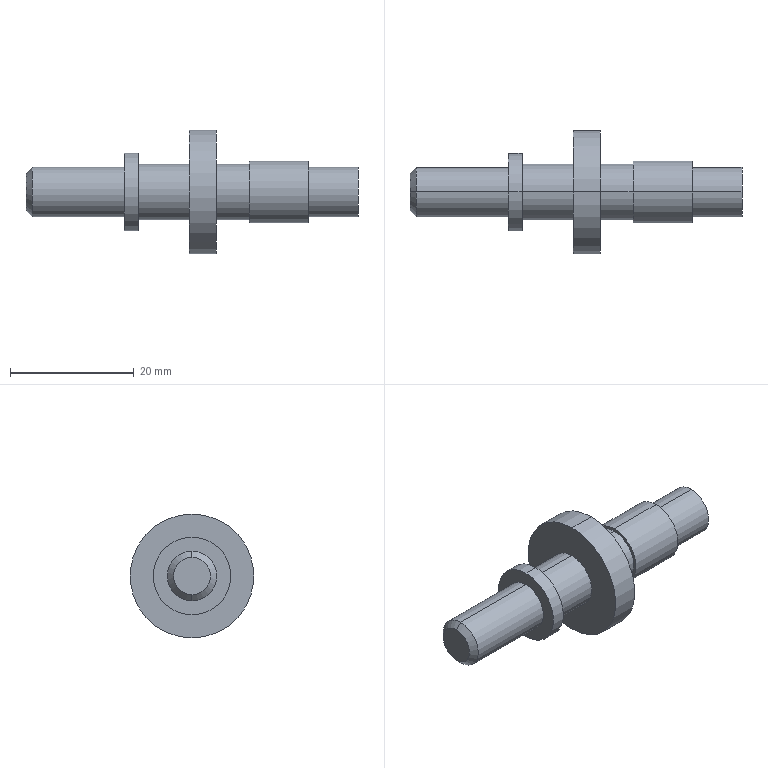Part | SolidWorks | features Revolution 1 | 1 solid | 25 faces | box 53.633 x 20 x 20 mm | volume 4453 mm3 | cylinder 14 | plane 7 | cone 4 | commonest cylinder face diameters 9 x4 8 x2 8.009 x2 10 x2 12.538 x2 20 x2
STEP:
#1=CARTESIAN_POINT('',(49.517,-18.474,-4.005));
#2=VERTEX_POINT('',#1);
#3=CARTESIAN_POINT('',(49.517,-18.474,4.005));
#4=VERTEX_POINT('',#3);
#5=CARTESIAN_POINT('',(49.517,-18.474,0.));
#6=DIRECTION('',(1.,0.,0.));
#7=DIRECTION('',(0.,0.,-1.));
#8=AXIS2_PLACEMENT_3D('',#5,#6,#7);
#9=CIRCLE('',#8,4.005);
#10=EDGE_CURVE('',#2,#4,#9,.T.);
#11=ORIENTED_EDGE('',*,*,#10,.F.);
#12=CARTESIAN_POINT('',(49.513,-18.474,-5.));
#13=VERTEX_POINT('',#12);
#14=CARTESIAN_POINT('',(49.517,-18.474,-4.005));
#15=DIRECTION('',(-0.003804,0.,-1.));
#16=VECTOR('',#15,1000.);
#17=LINE('',#14,#16);
#18=EDGE_CURVE('',#2,#13,#17,.T.);
#19=ORIENTED_EDGE('',*,*,#18,.T.);
#20=CARTESIAN_POINT('',(49.513,-18.474,5.));
#21=VERTEX_POINT('',#20);
#22=CARTESIAN_POINT('',(49.513,-18.474,0.));
#23=DIRECTION('',(1.,0.,0.));
#24=DIRECTION('',(0.,0.,-1.));
#25=AXIS2_PLACEMENT_3D('',#22,#23,#24);
#26=CIRCLE('',#25,5.);
#27=EDGE_CURVE('',#13,#21,#26,.T.);
#28=ORIENTED_EDGE('',*,*,#27,.T.);
#29=CARTESIAN_POINT('',(49.517,-18.474,4.005));
#30=DIRECTION('',(-0.003804,0.,1.));
#31=VECTOR('',#30,1000.);
#32=LINE('',#29,#31);
#33=EDGE_CURVE('',#4,#21,#32,.T.);
#34=ORIENTED_EDGE('',*,*,#33,.F.);
#35=EDGE_LOOP('',(#11,#19,#28,#34));
#36=FACE_OUTER_BOUND('',#35,.T.);
#37=CARTESIAN_POINT('',(49.517,-18.474,0.));
#38=DIRECTION('',(-1.,0.,0.));
#39=DIRECTION('',(0.,0.,1.));
#40=AXIS2_PLACEMENT_3D('',#37,#38,#39);
#41=CONICAL_SURFACE('',#40,4.005,1.567);
#42=ADVANCED_FACE('',(#36),#41,.T.);
#43=ORIENTED_EDGE('',*,*,#10,.T.);
#44=CARTESIAN_POINT('',(57.517,-18.474,4.005));
#45=VERTEX_POINT('',#44);
#46=CARTESIAN_POINT('',(3.884,-18.474,4.005));
#47=DIRECTION('',(1.,0.,0.));
#48=VECTOR('',#47,1000.);
#49=LINE('',#46,#48);
#50=EDGE_CURVE('',#4,#45,#49,.T.);
#51=ORIENTED_EDGE('',*,*,#50,.T.);
#52=CARTESIAN_POINT('',(57.517,-18.474,-4.005));
#53=VERTEX_POINT('',#52);
#54=CARTESIAN_POINT('',(57.517,-18.474,0.));
#55=DIRECTION('',(1.,0.,0.));
#56=DIRECTION('',(0.,0.,-1.));
#57=AXIS2_PLACEMENT_3D('',#54,#55,#56);
#58=CIRCLE('',#57,4.005);
#59=EDGE_CURVE('',#53,#45,#58,.T.);
#60=ORIENTED_EDGE('',*,*,#59,.F.);
#61=CARTESIAN_POINT('',(3.884,-18.474,-4.005));
#62=DIRECTION('',(1.,0.,0.));
#63=VECTOR('',#62,1000.);
#64=LINE('',#61,#63);
#65=EDGE_CURVE('',#2,#53,#64,.T.);
#66=ORIENTED_EDGE('',*,*,#65,.F.);
#67=EDGE_LOOP('',(#43,#51,#60,#66));
#68=FACE_OUTER_BOUND('',#67,.T.);
#69=CARTESIAN_POINT('',(3.884,-18.474,0.));
#70=DIRECTION('',(1.,0.,0.));
#71=DIRECTION('',(0.,0.,-1.));
#72=AXIS2_PLACEMENT_3D('',#69,#70,#71);
#73=CYLINDRICAL_SURFACE('',#72,4.005);
#74=ADVANCED_FACE('',(#68),#73,.T.);
#75=CARTESIAN_POINT('',(3.884,-18.474,-3.));
#76=VERTEX_POINT('',#75);
#77=CARTESIAN_POINT('',(3.884,-18.474,3.));
#78=VERTEX_POINT('',#77);
#79=CARTESIAN_POINT('',(3.884,-18.474,0.));
#80=DIRECTION('',(1.,0.,0.));
#81=DIRECTION('',(0.,0.,-1.));
#82=AXIS2_PLACEMENT_3D('',#79,#80,#81);
#83=CIRCLE('',#82,3.);
#84=EDGE_CURVE('',#76,#78,#83,.T.);
#85=ORIENTED_EDGE('',*,*,#84,.T.);
#86=CARTESIAN_POINT('',(4.884,-18.474,4.));
#87=VERTEX_POINT('',#86);
#88=CARTESIAN_POINT('',(4.884,-18.474,4.));
#89=DIRECTION('',(0.7071,0.,0.7071));
#90=VECTOR('',#89,1000.);
#91=LINE('',#88,#90);
#92=EDGE_CURVE('',#78,#87,#91,.T.);
#93=ORIENTED_EDGE('',*,*,#92,.T.);
#94=CARTESIAN_POINT('',(4.884,-18.474,-4.));
#95=VERTEX_POINT('',#94);
#96=CARTESIAN_POINT('',(4.884,-18.474,0.));
#97=DIRECTION('',(1.,0.,0.));
#98=DIRECTION('',(0.,0.,-1.));
#99=AXIS2_PLACEMENT_3D('',#96,#97,#98);
#100=CIRCLE('',#99,4.);
#101=EDGE_CURVE('',#95,#87,#100,.T.);
#102=ORIENTED_EDGE('',*,*,#101,.F.);
#103=CARTESIAN_POINT('',(4.884,-18.474,-4.));
#104=DIRECTION('',(0.7071,0.,-0.7071));
#105=VECTOR('',#104,1000.);
#106=LINE('',#103,#105);
#107=EDGE_CURVE('',#76,#95,#106,.T.);
#108=ORIENTED_EDGE('',*,*,#107,.F.);
#109=EDGE_LOOP('',(#85,#93,#102,#108));
#110=FACE_OUTER_BOUND('',#109,.T.);
#111=CARTESIAN_POINT('',(4.884,-18.474,0.));
#112=DIRECTION('',(1.,0.,0.));
#113=DIRECTION('',(0.,0.,-1.));
#114=AXIS2_PLACEMENT_3D('',#111,#112,#113);
#115=CONICAL_SURFACE('',#114,4.,0.7854);
#116=ADVANCED_FACE('',(#110),#115,.T.);
#117=ORIENTED_EDGE('',*,*,#101,.T.);
#118=CARTESIAN_POINT('',(19.769,-18.474,4.));
#119=VERTEX_POINT('',#118);
#120=CARTESIAN_POINT('',(3.884,-18.474,4.));
#121=DIRECTION('',(1.,0.,0.));
#122=VECTOR('',#121,1000.);
#123=LINE('',#120,#122);
#124=EDGE_CURVE('',#87,#119,#123,.T.);
#125=ORIENTED_EDGE('',*,*,#124,.T.);
#126=CARTESIAN_POINT('',(19.769,-18.474,-4.));
#127=VERTEX_POINT('',#126);
#128=CARTESIAN_POINT('',(19.769,-18.474,0.));
#129=DIRECTION('',(1.,0.,0.));
#130=DIRECTION('',(0.,0.,-1.));
#131=AXIS2_PLACEMENT_3D('',#128,#129,#130);
#132=CIRCLE('',#131,4.);
#133=EDGE_CURVE('',#127,#119,#132,.T.);
#134=ORIENTED_EDGE('',*,*,#133,.F.);
#135=CARTESIAN_POINT('',(3.884,-18.474,-4.));
#136=DIRECTION('',(1.,0.,0.));
#137=VECTOR('',#136,1000.);
#138=LINE('',#135,#137);
#139=EDGE_CURVE('',#95,#127,#138,.T.);
#140=ORIENTED_EDGE('',*,*,#139,.F.);
#141=EDGE_LOOP('',(#117,#125,#134,#140));
#142=FACE_OUTER_BOUND('',#141,.T.);
#143=CARTESIAN_POINT('',(3.884,-18.474,0.));
#144=DIRECTION('',(1.,0.,0.));
#145=DIRECTION('',(0.,0.,-1.));
#146=AXIS2_PLACEMENT_3D('',#143,#144,#145);
#147=CYLINDRICAL_SURFACE('',#146,4.);
#148=ADVANCED_FACE('',(#142),#147,.T.);
#149=CARTESIAN_POINT('',(19.769,-18.474,-6.269));
#150=VERTEX_POINT('',#149);
#151=CARTESIAN_POINT('',(19.769,-18.474,6.269));
#152=VERTEX_POINT('',#151);
#153=CARTESIAN_POINT('',(19.769,-18.474,0.));
#154=DIRECTION('',(1.,0.,0.));
#155=DIRECTION('',(0.,0.,-1.));
#156=AXIS2_PLACEMENT_3D('',#153,#154,#155);
#157=CIRCLE('',#156,6.269);
#158=EDGE_CURVE('',#150,#152,#157,.T.);
#159=ORIENTED_EDGE('',*,*,#158,.T.);
#160=CARTESIAN_POINT('',(22.015,-18.474,6.269));
#161=VERTEX_POINT('',#160);
#162=CARTESIAN_POINT('',(3.884,-18.474,6.269));
#163=DIRECTION('',(1.,0.,0.));
#164=VECTOR('',#163,1000.);
#165=LINE('',#162,#164);
#166=EDGE_CURVE('',#152,#161,#165,.T.);
#167=ORIENTED_EDGE('',*,*,#166,.T.);
#168=CARTESIAN_POINT('',(22.015,-18.474,-6.269));
#169=VERTEX_POINT('',#168);
#170=CARTESIAN_POINT('',(22.015,-18.474,0.));
#171=DIRECTION('',(1.,0.,0.));
#172=DIRECTION('',(0.,0.,-1.));
#173=AXIS2_PLACEMENT_3D('',#170,#171,#172);
#174=CIRCLE('',#173,6.269);
#175=EDGE_CURVE('',#169,#161,#174,.T.);
#176=ORIENTED_EDGE('',*,*,#175,.F.);
#177=CARTESIAN_POINT('',(3.884,-18.474,-6.269));
#178=DIRECTION('',(1.,0.,0.));
#179=VECTOR('',#178,1000.);
#180=LINE('',#177,#179);
#181=EDGE_CURVE('',#150,#169,#180,.T.);
#182=ORIENTED_EDGE('',*,*,#181,.F.);
#183=EDGE_LOOP('',(#159,#167,#176,#182));
#184=FACE_OUTER_BOUND('',#183,.T.);
#185=CARTESIAN_POINT('',(3.884,-18.474,0.));
#186=DIRECTION('',(1.,0.,0.));
#187=DIRECTION('',(0.,0.,-1.));
#188=AXIS2_PLACEMENT_3D('',#185,#186,#187);
#189=CYLINDRICAL_SURFACE('',#188,6.269);
#190=ADVANCED_FACE('',(#184),#189,.T.);
#191=CARTESIAN_POINT('',(22.015,-18.474,-4.5));
#192=VERTEX_POINT('',#191);
#193=CARTESIAN_POINT('',(22.015,-18.474,4.5));
#194=VERTEX_POINT('',#193);
#195=CARTESIAN_POINT('',(22.015,-18.474,0.));
#196=DIRECTION('',(1.,0.,0.));
#197=DIRECTION('',(0.,0.,-1.));
#198=AXIS2_PLACEMENT_3D('',#195,#196,#197);
#199=CIRCLE('',#198,4.5);
#200=EDGE_CURVE('',#192,#194,#199,.T.);
#201=ORIENTED_EDGE('',*,*,#200,.T.);
#202=CARTESIAN_POINT('',(30.281,-18.474,4.5));
#203=VERTEX_POINT('',#202);
#204=CARTESIAN_POINT('',(3.884,-18.474,4.5));
#205=DIRECTION('',(1.,0.,0.));
#206=VECTOR('',#205,1000.);
#207=LINE('',#204,#206);
#208=EDGE_CURVE('',#194,#203,#207,.T.);
#209=ORIENTED_EDGE('',*,*,#208,.T.);
#210=CARTESIAN_POINT('',(30.281,-18.474,-4.5));
#211=VERTEX_POINT('',#210);
#212=CARTESIAN_POINT('',(30.281,-18.474,0.));
#213=DIRECTION('',(1.,0.,0.));
#214=DIRECTION('',(0.,0.,-1.));
#215=AXIS2_PLACEMENT_3D('',#212,#213,#214);
#216=CIRCLE('',#215,4.5);
#217=EDGE_CURVE('',#211,#203,#216,.T.);
#218=ORIENTED_EDGE('',*,*,#217,.F.);
#219=CARTESIAN_POINT('',(3.884,-18.474,-4.5));
#220=DIRECTION('',(1.,0.,0.));
#221=VECTOR('',#220,1000.);
#222=LINE('',#219,#221);
#223=EDGE_CURVE('',#192,#211,#222,.T.);
#224=ORIENTED_EDGE('',*,*,#223,.F.);
#225=EDGE_LOOP('',(#201,#209,#218,#224));
#226=FACE_OUTER_BOUND('',#225,.T.);
#227=CARTESIAN_POINT('',(3.884,-18.474,0.));
#228=DIRECTION('',(1.,0.,0.));
#229=DIRECTION('',(0.,0.,-1.));
#230=AXIS2_PLACEMENT_3D('',#227,#228,#229);
#231=CYLINDRICAL_SURFACE('',#230,4.5);
#232=ADVANCED_FACE('',(#226),#231,.T.);
#233=CARTESIAN_POINT('',(30.281,-18.474,-10.));
#234=VERTEX_POINT('',#233);
#235=CARTESIAN_POINT('',(30.281,-18.474,10.));
#236=VERTEX_POINT('',#235);
#237=CARTESIAN_POINT('',(30.281,-18.474,0.));
#238=DIRECTION('',(1.,0.,0.));
#239=DIRECTION('',(0.,0.,-1.));
#240=AXIS2_PLACEMENT_3D('',#237,#238,#239);
#241=CIRCLE('',#240,10.);
#242=EDGE_CURVE('',#234,#236,#241,.T.);
#243=ORIENTED_EDGE('',*,*,#242,.T.);
#244=CARTESIAN_POINT('',(34.643,-18.474,10.));
#245=VERTEX_POINT('',#244);
#246=CARTESIAN_POINT('',(3.884,-18.474,10.));
#247=DIRECTION('',(1.,0.,0.));
#248=VECTOR('',#247,1000.);
#249=LINE('',#246,#248);
#250=EDGE_CURVE('',#236,#245,#249,.T.);
#251=ORIENTED_EDGE('',*,*,#250,.T.);
#252=CARTESIAN_POINT('',(34.643,-18.474,-10.));
#253=VERTEX_POINT('',#252);
#254=CARTESIAN_POINT('',(34.643,-18.474,0.));
#255=DIRECTION('',(1.,0.,0.));
#256=DIRECTION('',(0.,0.,-1.));
#257=AXIS2_PLACEMENT_3D('',#254,#255,#256);
#258=CIRCLE('',#257,10.);
#259=EDGE_CURVE('',#253,#245,#258,.T.);
#260=ORIENTED_EDGE('',*,*,#259,.F.);
#261=CARTESIAN_POINT('',(3.884,-18.474,-10.));
#262=DIRECTION('',(1.,0.,0.));
#263=VECTOR('',#262,1000.);
#264=LINE('',#261,#263);
#265=EDGE_CURVE('',#234,#253,#264,.T.);
#266=ORIENTED_EDGE('',*,*,#265,.F.);
#267=EDGE_LOOP('',(#243,#251,#260,#266));
#268=FACE_OUTER_BOUND('',#267,.T.);
#269=CARTESIAN_POINT('',(3.884,-18.474,0.));
#270=DIRECTION('',(1.,0.,0.));
#271=DIRECTION('',(0.,0.,-1.));
#272=AXIS2_PLACEMENT_3D('',#269,#270,#271);
#273=CYLINDRICAL_SURFACE('',#272,10.);
#274=ADVANCED_FACE('',(#268),#273,.T.);
#275=CARTESIAN_POINT('',(34.643,-18.474,-4.5));
#276=VERTEX_POINT('',#275);
#277=CARTESIAN_POINT('',(34.643,-18.474,4.5));
#278=VERTEX_POINT('',#277);
#279=CARTESIAN_POINT('',(34.643,-18.474,0.));
#280=DIRECTION('',(1.,0.,0.));
#281=DIRECTION('',(0.,0.,-1.));
#282=AXIS2_PLACEMENT_3D('',#279,#280,#281);
#283=CIRCLE('',#282,4.5);
#284=EDGE_CURVE('',#276,#278,#283,.T.);
#285=ORIENTED_EDGE('',*,*,#284,.T.);
#286=CARTESIAN_POINT('',(39.924,-18.474,4.5));
#287=VERTEX_POINT('',#286);
#288=CARTESIAN_POINT('',(3.884,-18.474,4.5));
#289=DIRECTION('',(1.,0.,0.));
#290=VECTOR('',#289,1000.);
#291=LINE('',#288,#290);
#292=EDGE_CURVE('',#278,#287,#291,.T.);
#293=ORIENTED_EDGE('',*,*,#292,.T.);
#294=CARTESIAN_POINT('',(39.924,-18.474,-4.5));
#295=VERTEX_POINT('',#294);
#296=CARTESIAN_POINT('',(39.924,-18.474,0.));
#297=DIRECTION('',(1.,0.,0.));
#298=DIRECTION('',(0.,0.,-1.));
#299=AXIS2_PLACEMENT_3D('',#296,#297,#298);
#300=CIRCLE('',#299,4.5);
#301=EDGE_CURVE('',#295,#287,#300,.T.);
#302=ORIENTED_EDGE('',*,*,#301,.F.);
#303=CARTESIAN_POINT('',(3.884,-18.474,-4.5));
#304=DIRECTION('',(1.,0.,0.));
#305=VECTOR('',#304,1000.);
#306=LINE('',#303,#305);
#307=EDGE_CURVE('',#276,#295,#306,.T.);
#308=ORIENTED_EDGE('',*,*,#307,.F.);
#309=EDGE_LOOP('',(#285,#293,#302,#308));
#310=FACE_OUTER_BOUND('',#309,.T.);
#311=CARTESIAN_POINT('',(3.884,-18.474,0.));
#312=DIRECTION('',(1.,0.,0.));
#313=DIRECTION('',(0.,0.,-1.));
#314=AXIS2_PLACEMENT_3D('',#311,#312,#313);
#315=CYLINDRICAL_SURFACE('',#314,4.5);
#316=ADVANCED_FACE('',(#310),#315,.T.);
#317=CARTESIAN_POINT('',(39.924,-18.474,-5.));
#318=VERTEX_POINT('',#317);
#319=CARTESIAN_POINT('',(39.924,-18.474,5.));
#320=VERTEX_POINT('',#319);
#321=CARTESIAN_POINT('',(39.924,-18.474,0.));
#322=DIRECTION('',(1.,0.,0.));
#323=DIRECTION('',(0.,0.,-1.));
#324=AXIS2_PLACEMENT_3D('',#321,#322,#323);
#325=CIRCLE('',#324,5.);
#326=EDGE_CURVE('',#318,#320,#325,.T.);
#327=ORIENTED_EDGE('',*,*,#326,.T.);
#328=CARTESIAN_POINT('',(3.884,-18.474,5.));
#329=DIRECTION('',(1.,0.,0.));
#330=VECTOR('',#329,1000.);
#331=LINE('',#328,#330);
#332=EDGE_CURVE('',#320,#21,#331,.T.);
#333=ORIENTED_EDGE('',*,*,#332,.T.);
#334=ORIENTED_EDGE('',*,*,#27,.F.);
#335=CARTESIAN_POINT('',(3.884,-18.474,-5.));
#336=DIRECTION('',(1.,0.,0.));
#337=VECTOR('',#336,1000.);
#338=LINE('',#335,#337);
#339=EDGE_CURVE('',#318,#13,#338,.T.);
#340=ORIENTED_EDGE('',*,*,#339,.F.);
#341=EDGE_LOOP('',(#327,#333,#334,#340));
#342=FACE_OUTER_BOUND('',#341,.T.);
#343=CARTESIAN_POINT('',(3.884,-18.474,0.));
#344=DIRECTION('',(1.,0.,0.));
#345=DIRECTION('',(0.,0.,-1.));
#346=AXIS2_PLACEMENT_3D('',#343,#344,#345);
#347=CYLINDRICAL_SURFACE('',#346,5.);
#348=ADVANCED_FACE('',(#342),#347,.T.);
#349=ORIENTED_EDGE('',*,*,#332,.F.);
#350=CARTESIAN_POINT('',(39.924,-18.474,0.));
#351=DIRECTION('',(1.,0.,0.));
#352=DIRECTION('',(0.,0.,-1.));
#353=AXIS2_PLACEMENT_3D('',#350,#351,#352);
#354=CIRCLE('',#353,5.);
#355=EDGE_CURVE('',#320,#318,#354,.T.);
#356=ORIENTED_EDGE('',*,*,#355,.T.);
#357=ORIENTED_EDGE('',*,*,#339,.T.);
#358=CARTESIAN_POINT('',(49.513,-18.474,0.));
#359=DIRECTION('',(1.,0.,0.));
#360=DIRECTION('',(0.,0.,-1.));
#361=AXIS2_PLACEMENT_3D('',#358,#359,#360);
#362=CIRCLE('',#361,5.);
#363=EDGE_CURVE('',#21,#13,#362,.T.);
#364=ORIENTED_EDGE('',*,*,#363,.F.);
#365=EDGE_LOOP('',(#349,#356,#357,#364));
#366=FACE_OUTER_BOUND('',#365,.T.);
#367=CARTESIAN_POINT('',(3.884,-18.474,0.));
#368=DIRECTION('',(1.,0.,0.));
#369=DIRECTION('',(0.,0.,-1.));
#370=AXIS2_PLACEMENT_3D('',#367,#368,#369);
#371=CYLINDRICAL_SURFACE('',#370,5.);
#372=ADVANCED_FACE('',(#366),#371,.T.);
#373=ORIENTED_EDGE('',*,*,#301,.T.);
#374=CARTESIAN_POINT('',(39.924,-18.474,0.));
#375=DIRECTION('',(1.,0.,0.));
#376=DIRECTION('',(0.,0.,-1.));
#377=AXIS2_PLACEMENT_3D('',#374,#375,#376);
#378=CIRCLE('',#377,4.5);
#379=EDGE_CURVE('',#287,#295,#378,.T.);
#380=ORIENTED_EDGE('',*,*,#379,.T.);
#381=EDGE_LOOP('',(#373,#380));
#382=FACE_BOUND('',#381,.T.);
#383=ORIENTED_EDGE('',*,*,#326,.F.);
#384=ORIENTED_EDGE('',*,*,#355,.F.);
#385=EDGE_LOOP('',(#383,#384));
#386=FACE_OUTER_BOUND('',#385,.T.);
#387=CARTESIAN_POINT('',(39.924,-13.474,0.));
#388=DIRECTION('',(-1.,0.,0.));
#389=DIRECTION('',(0.,0.,1.));
#390=AXIS2_PLACEMENT_3D('',#387,#388,#389);
#391=PLANE('',#390);
#392=ADVANCED_FACE('',(#382,#386),#391,.T.);
#393=ORIENTED_EDGE('',*,*,#292,.F.);
#394=CARTESIAN_POINT('',(34.643,-18.474,0.));
#395=DIRECTION('',(1.,0.,0.));
#396=DIRECTION('',(0.,0.,-1.));
#397=AXIS2_PLACEMENT_3D('',#394,#395,#396);
#398=CIRCLE('',#397,4.5);
#399=EDGE_CURVE('',#278,#276,#398,.T.);
#400=ORIENTED_EDGE('',*,*,#399,.T.);
#401=ORIENTED_EDGE('',*,*,#307,.T.);
#402=ORIENTED_EDGE('',*,*,#379,.F.);
#403=EDGE_LOOP('',(#393,#400,#401,#402));
#404=FACE_OUTER_BOUND('',#403,.T.);
#405=CARTESIAN_POINT('',(3.884,-18.474,0.));
#406=DIRECTION('',(1.,0.,0.));
#407=DIRECTION('',(0.,0.,-1.));
#408=AXIS2_PLACEMENT_3D('',#405,#406,#407);
#409=CYLINDRICAL_SURFACE('',#408,4.5);
#410=ADVANCED_FACE('',(#404),#409,.T.);
#411=ORIENTED_EDGE('',*,*,#259,.T.);
#412=CARTESIAN_POINT('',(34.643,-18.474,0.));
#413=DIRECTION('',(1.,0.,0.));
#414=DIRECTION('',(0.,0.,-1.));
#415=AXIS2_PLACEMENT_3D('',#412,#413,#414);
#416=CIRCLE('',#415,10.);
#417=EDGE_CURVE('',#245,#253,#416,.T.);
#418=ORIENTED_EDGE('',*,*,#417,.T.);
#419=EDGE_LOOP('',(#411,#418));
#420=FACE_OUTER_BOUND('',#419,.T.);
#421=ORIENTED_EDGE('',*,*,#284,.F.);
#422=ORIENTED_EDGE('',*,*,#399,.F.);
#423=EDGE_LOOP('',(#421,#422));
#424=FACE_BOUND('',#423,.T.);
#425=CARTESIAN_POINT('',(34.643,-13.974,0.));
#426=DIRECTION('',(1.,0.,0.));
#427=DIRECTION('',(0.,0.,-1.));
#428=AXIS2_PLACEMENT_3D('',#425,#426,#427);
#429=PLANE('',#428);
#430=ADVANCED_FACE('',(#420,#424),#429,.T.);
#431=ORIENTED_EDGE('',*,*,#250,.F.);
#432=CARTESIAN_POINT('',(30.281,-18.474,0.));
#433=DIRECTION('',(1.,0.,0.));
#434=DIRECTION('',(0.,0.,-1.));
#435=AXIS2_PLACEMENT_3D('',#432,#433,#434);
#436=CIRCLE('',#435,10.);
#437=EDGE_CURVE('',#236,#234,#436,.T.);
#438=ORIENTED_EDGE('',*,*,#437,.T.);
#439=ORIENTED_EDGE('',*,*,#265,.T.);
#440=ORIENTED_EDGE('',*,*,#417,.F.);
#441=EDGE_LOOP('',(#431,#438,#439,#440));
#442=FACE_OUTER_BOUND('',#441,.T.);
#443=CARTESIAN_POINT('',(3.884,-18.474,0.));
#444=DIRECTION('',(1.,0.,0.));
#445=DIRECTION('',(0.,0.,-1.));
#446=AXIS2_PLACEMENT_3D('',#443,#444,#445);
#447=CYLINDRICAL_SURFACE('',#446,10.);
#448=ADVANCED_FACE('',(#442),#447,.T.);
#449=ORIENTED_EDGE('',*,*,#217,.T.);
#450=CARTESIAN_POINT('',(30.281,-18.474,0.));
#451=DIRECTION('',(1.,0.,0.));
#452=DIRECTION('',(0.,0.,-1.));
#453=AXIS2_PLACEMENT_3D('',#450,#451,#452);
#454=CIRCLE('',#453,4.5);
#455=EDGE_CURVE('',#203,#211,#454,.T.);
#456=ORIENTED_EDGE('',*,*,#455,.T.);
#457=EDGE_LOOP('',(#449,#456));
#458=FACE_BOUND('',#457,.T.);
#459=ORIENTED_EDGE('',*,*,#242,.F.);
#460=ORIENTED_EDGE('',*,*,#437,.F.);
#461=EDGE_LOOP('',(#459,#460));
#462=FACE_OUTER_BOUND('',#461,.T.);
#463=CARTESIAN_POINT('',(30.281,-8.474,0.));
#464=DIRECTION('',(-1.,0.,0.));
#465=DIRECTION('',(0.,0.,1.));
#466=AXIS2_PLACEMENT_3D('',#463,#464,#465);
#467=PLANE('',#466);
#468=ADVANCED_FACE('',(#458,#462),#467,.T.);
#469=ORIENTED_EDGE('',*,*,#208,.F.);
#470=CARTESIAN_POINT('',(22.015,-18.474,0.));
#471=DIRECTION('',(1.,0.,0.));
#472=DIRECTION('',(0.,0.,-1.));
#473=AXIS2_PLACEMENT_3D('',#470,#471,#472);
#474=CIRCLE('',#473,4.5);
#475=EDGE_CURVE('',#194,#192,#474,.T.);
#476=ORIENTED_EDGE('',*,*,#475,.T.);
#477=ORIENTED_EDGE('',*,*,#223,.T.);
#478=ORIENTED_EDGE('',*,*,#455,.F.);
#479=EDGE_LOOP('',(#469,#476,#477,#478));
#480=FACE_OUTER_BOUND('',#479,.T.);
#481=CARTESIAN_POINT('',(3.884,-18.474,0.));
#482=DIRECTION('',(1.,0.,0.));
#483=DIRECTION('',(0.,0.,-1.));
#484=AXIS2_PLACEMENT_3D('',#481,#482,#483);
#485=CYLINDRICAL_SURFACE('',#484,4.5);
#486=ADVANCED_FACE('',(#480),#485,.T.);
#487=ORIENTED_EDGE('',*,*,#175,.T.);
#488=CARTESIAN_POINT('',(22.015,-18.474,0.));
#489=DIRECTION('',(1.,0.,0.));
#490=DIRECTION('',(0.,0.,-1.));
#491=AXIS2_PLACEMENT_3D('',#488,#489,#490);
#492=CIRCLE('',#491,6.269);
#493=EDGE_CURVE('',#161,#169,#492,.T.);
#494=ORIENTED_EDGE('',*,*,#493,.T.);
#495=EDGE_LOOP('',(#487,#494));
#496=FACE_OUTER_BOUND('',#495,.T.);
#497=ORIENTED_EDGE('',*,*,#200,.F.);
#498=ORIENTED_EDGE('',*,*,#475,.F.);
#499=EDGE_LOOP('',(#497,#498));
#500=FACE_BOUND('',#499,.T.);
#501=CARTESIAN_POINT('',(22.015,-12.205,0.));
#502=DIRECTION('',(1.,0.,0.));
#503=DIRECTION('',(0.,0.,-1.));
#504=AXIS2_PLACEMENT_3D('',#501,#502,#503);
#505=PLANE('',#504);
#506=ADVANCED_FACE('',(#496,#500),#505,.T.);
#507=ORIENTED_EDGE('',*,*,#166,.F.);
#508=CARTESIAN_POINT('',(19.769,-18.474,0.));
#509=DIRECTION('',(1.,0.,0.));
#510=DIRECTION('',(0.,0.,-1.));
#511=AXIS2_PLACEMENT_3D('',#508,#509,#510);
#512=CIRCLE('',#511,6.269);
#513=EDGE_CURVE('',#152,#150,#512,.T.);
#514=ORIENTED_EDGE('',*,*,#513,.T.);
#515=ORIENTED_EDGE('',*,*,#181,.T.);
#516=ORIENTED_EDGE('',*,*,#493,.F.);
#517=EDGE_LOOP('',(#507,#514,#515,#516));
#518=FACE_OUTER_BOUND('',#517,.T.);
#519=CARTESIAN_POINT('',(3.884,-18.474,0.));
#520=DIRECTION('',(1.,0.,0.));
#521=DIRECTION('',(0.,0.,-1.));
#522=AXIS2_PLACEMENT_3D('',#519,#520,#521);
#523=CYLINDRICAL_SURFACE('',#522,6.269);
#524=ADVANCED_FACE('',(#518),#523,.T.);
#525=ORIENTED_EDGE('',*,*,#133,.T.);
#526=CARTESIAN_POINT('',(19.769,-18.474,0.));
#527=DIRECTION('',(1.,0.,0.));
#528=DIRECTION('',(0.,0.,-1.));
#529=AXIS2_PLACEMENT_3D('',#526,#527,#528);
#530=CIRCLE('',#529,4.);
#531=EDGE_CURVE('',#119,#127,#530,.T.);
#532=ORIENTED_EDGE('',*,*,#531,.T.);
#533=EDGE_LOOP('',(#525,#532));
#534=FACE_BOUND('',#533,.T.);
#535=ORIENTED_EDGE('',*,*,#158,.F.);
#536=ORIENTED_EDGE('',*,*,#513,.F.);
#537=EDGE_LOOP('',(#535,#536));
#538=FACE_OUTER_BOUND('',#537,.T.);
#539=CARTESIAN_POINT('',(19.769,-12.205,0.));
#540=DIRECTION('',(-1.,0.,0.));
#541=DIRECTION('',(0.,0.,1.));
#542=AXIS2_PLACEMENT_3D('',#539,#540,#541);
#543=PLANE('',#542);
#544=ADVANCED_FACE('',(#534,#538),#543,.T.);
#545=ORIENTED_EDGE('',*,*,#124,.F.);
#546=CARTESIAN_POINT('',(4.884,-18.474,0.));
#547=DIRECTION('',(1.,0.,0.));
#548=DIRECTION('',(0.,0.,-1.));
#549=AXIS2_PLACEMENT_3D('',#546,#547,#548);
#550=CIRCLE('',#549,4.);
#551=EDGE_CURVE('',#87,#95,#550,.T.);
#552=ORIENTED_EDGE('',*,*,#551,.T.);
#553=ORIENTED_EDGE('',*,*,#139,.T.);
#554=ORIENTED_EDGE('',*,*,#531,.F.);
#555=EDGE_LOOP('',(#545,#552,#553,#554));
#556=FACE_OUTER_BOUND('',#555,.T.);
#557=CARTESIAN_POINT('',(3.884,-18.474,0.));
#558=DIRECTION('',(1.,0.,0.));
#559=DIRECTION('',(0.,0.,-1.));
#560=AXIS2_PLACEMENT_3D('',#557,#558,#559);
#561=CYLINDRICAL_SURFACE('',#560,4.);
#562=ADVANCED_FACE('',(#556),#561,.T.);
#563=ORIENTED_EDGE('',*,*,#92,.F.);
#564=CARTESIAN_POINT('',(3.884,-18.474,0.));
#565=DIRECTION('',(1.,0.,0.));
#566=DIRECTION('',(0.,0.,-1.));
#567=AXIS2_PLACEMENT_3D('',#564,#565,#566);
#568=CIRCLE('',#567,3.);
#569=EDGE_CURVE('',#78,#76,#568,.T.);
#570=ORIENTED_EDGE('',*,*,#569,.T.);
#571=ORIENTED_EDGE('',*,*,#107,.T.);
#572=ORIENTED_EDGE('',*,*,#551,.F.);
#573=EDGE_LOOP('',(#563,#570,#571,#572));
#574=FACE_OUTER_BOUND('',#573,.T.);
#575=CARTESIAN_POINT('',(4.884,-18.474,0.));
#576=DIRECTION('',(1.,0.,0.));
#577=DIRECTION('',(0.,0.,-1.));
#578=AXIS2_PLACEMENT_3D('',#575,#576,#577);
#579=CONICAL_SURFACE('',#578,4.,0.7854);
#580=ADVANCED_FACE('',(#574),#579,.T.);
#581=ORIENTED_EDGE('',*,*,#84,.F.);
#582=ORIENTED_EDGE('',*,*,#569,.F.);
#583=EDGE_LOOP('',(#581,#582));
#584=FACE_OUTER_BOUND('',#583,.T.);
#585=CARTESIAN_POINT('',(3.884,-15.474,0.));
#586=DIRECTION('',(-1.,0.,0.));
#587=DIRECTION('',(0.,0.,1.));
#588=AXIS2_PLACEMENT_3D('',#585,#586,#587);
#589=PLANE('',#588);
#590=ADVANCED_FACE('',(#584),#589,.T.);
#591=ORIENTED_EDGE('',*,*,#59,.T.);
#592=CARTESIAN_POINT('',(57.517,-18.474,0.));
#593=DIRECTION('',(1.,0.,0.));
#594=DIRECTION('',(0.,0.,-1.));
#595=AXIS2_PLACEMENT_3D('',#592,#593,#594);
#596=CIRCLE('',#595,4.005);
#597=EDGE_CURVE('',#45,#53,#596,.T.);
#598=ORIENTED_EDGE('',*,*,#597,.T.);
#599=EDGE_LOOP('',(#591,#598));
#600=FACE_OUTER_BOUND('',#599,.T.);
#601=CARTESIAN_POINT('',(57.517,-18.474,0.));
#602=DIRECTION('',(1.,0.,0.));
#603=DIRECTION('',(0.,0.,-1.));
#604=AXIS2_PLACEMENT_3D('',#601,#602,#603);
#605=PLANE('',#604);
#606=ADVANCED_FACE('',(#600),#605,.T.);
#607=ORIENTED_EDGE('',*,*,#50,.F.);
#608=CARTESIAN_POINT('',(49.517,-18.474,0.));
#609=DIRECTION('',(1.,0.,0.));
#610=DIRECTION('',(0.,0.,-1.));
#611=AXIS2_PLACEMENT_3D('',#608,#609,#610);
#612=CIRCLE('',#611,4.005);
#613=EDGE_CURVE('',#4,#2,#612,.T.);
#614=ORIENTED_EDGE('',*,*,#613,.T.);
#615=ORIENTED_EDGE('',*,*,#65,.T.);
#616=ORIENTED_EDGE('',*,*,#597,.F.);
#617=EDGE_LOOP('',(#607,#614,#615,#616));
#618=FACE_OUTER_BOUND('',#617,.T.);
#619=CARTESIAN_POINT('',(3.884,-18.474,0.));
#620=DIRECTION('',(1.,0.,0.));
#621=DIRECTION('',(0.,0.,-1.));
#622=AXIS2_PLACEMENT_3D('',#619,#620,#621);
#623=CYLINDRICAL_SURFACE('',#622,4.005);
#624=ADVANCED_FACE('',(#618),#623,.T.);
#625=ORIENTED_EDGE('',*,*,#18,.F.);
#626=ORIENTED_EDGE('',*,*,#613,.F.);
#627=ORIENTED_EDGE('',*,*,#33,.T.);
#628=ORIENTED_EDGE('',*,*,#363,.T.);
#629=EDGE_LOOP('',(#625,#626,#627,#628));
#630=FACE_OUTER_BOUND('',#629,.T.);
#631=CARTESIAN_POINT('',(49.517,-18.474,0.));
#632=DIRECTION('',(-1.,0.,0.));
#633=DIRECTION('',(0.,0.,1.));
#634=AXIS2_PLACEMENT_3D('',#631,#632,#633);
#635=CONICAL_SURFACE('',#634,4.005,1.567);
#636=ADVANCED_FACE('',(#630),#635,.T.);
#637=CLOSED_SHELL('',(#42,#74,#116,#148,#190,#232,#274,#316,#348,#372,#392,#410,#430,#448,#468,#486,#506,#524,#544,#562,#580,#590,#606,#624,#636));
#638=MANIFOLD_SOLID_BREP('',#637);
#639=CARTESIAN_POINT('',(0.,0.,0.));
#640=DIRECTION('',(0.,0.,1.));
#641=DIRECTION('',(1.,0.,0.));
#642=AXIS2_PLACEMENT_3D('',#639,#640,#641);
#643=(LENGTH_UNIT()NAMED_UNIT(*)SI_UNIT(.MILLI.,.METRE.));
#644=UNCERTAINTY_MEASURE_WITH_UNIT(LENGTH_MEASURE(0.00001),#643,'','');
#645=(NAMED_UNIT(*)PLANE_ANGLE_UNIT()SI_UNIT($,.RADIAN.));
#646=(NAMED_UNIT(*)SI_UNIT($,.STERADIAN.)SOLID_ANGLE_UNIT());
#647=(GEOMETRIC_REPRESENTATION_CONTEXT(3)GLOBAL_UNCERTAINTY_ASSIGNED_CONTEXT((#644))GLOBAL_UNIT_ASSIGNED_CONTEXT((#643,#645,#646))REPRESENTATION_CONTEXT('',''));
#648=ADVANCED_BREP_SHAPE_REPRESENTATION('',(#638,#642),#647);